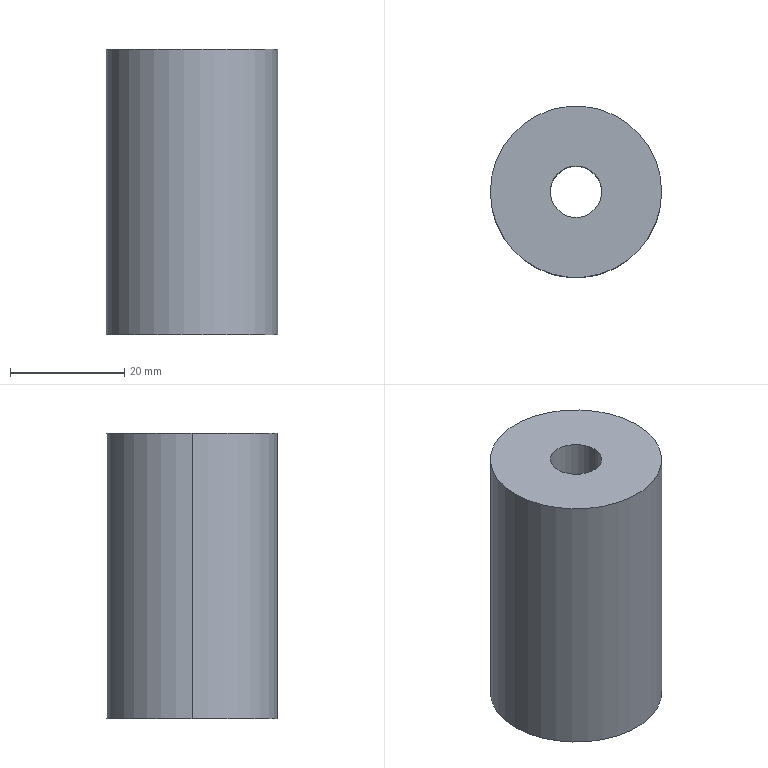Part | SolidWorks | features Extrusion 1 | 1 solid | 6 faces | box 30 x 30 x 50 mm | volume 32162 mm3 | cylinder 4 | plane 2 | commonest cylinder face diameters 9 x2 30 x2
STEP:
#1=CARTESIAN_POINT('',(-4.5,0.,50.));
#2=VERTEX_POINT('',#1);
#3=CARTESIAN_POINT('',(4.5,0.,50.));
#4=VERTEX_POINT('',#3);
#5=CARTESIAN_POINT('',(0.,0.,50.));
#6=DIRECTION('',(0.,0.,1.));
#7=DIRECTION('',(1.,0.,0.));
#8=AXIS2_PLACEMENT_3D('',#5,#6,#7);
#9=CIRCLE('',#8,4.5);
#10=EDGE_CURVE('',#2,#4,#9,.T.);
#11=ORIENTED_EDGE('',*,*,#10,.T.);
#12=CARTESIAN_POINT('',(4.5,0.,0.));
#13=VERTEX_POINT('',#12);
#14=CARTESIAN_POINT('',(4.5,0.,50.));
#15=DIRECTION('',(0.,0.,-1.));
#16=VECTOR('',#15,1000.);
#17=LINE('',#14,#16);
#18=EDGE_CURVE('',#4,#13,#17,.T.);
#19=ORIENTED_EDGE('',*,*,#18,.T.);
#20=CARTESIAN_POINT('',(-4.5,0.,0.));
#21=VERTEX_POINT('',#20);
#22=CARTESIAN_POINT('',(0.,0.,0.));
#23=DIRECTION('',(0.,0.,1.));
#24=DIRECTION('',(1.,0.,0.));
#25=AXIS2_PLACEMENT_3D('',#22,#23,#24);
#26=CIRCLE('',#25,4.5);
#27=EDGE_CURVE('',#21,#13,#26,.T.);
#28=ORIENTED_EDGE('',*,*,#27,.F.);
#29=CARTESIAN_POINT('',(-4.5,0.,50.));
#30=DIRECTION('',(0.,0.,-1.));
#31=VECTOR('',#30,1000.);
#32=LINE('',#29,#31);
#33=EDGE_CURVE('',#2,#21,#32,.T.);
#34=ORIENTED_EDGE('',*,*,#33,.F.);
#35=EDGE_LOOP('',(#11,#19,#28,#34));
#36=FACE_OUTER_BOUND('',#35,.T.);
#37=CARTESIAN_POINT('',(0.,0.,50.));
#38=DIRECTION('',(0.,0.,-1.));
#39=DIRECTION('',(-1.,0.,0.));
#40=AXIS2_PLACEMENT_3D('',#37,#38,#39);
#41=CYLINDRICAL_SURFACE('',#40,4.5);
#42=ADVANCED_FACE('',(#36),#41,.F.);
#43=CARTESIAN_POINT('',(15.,0.,50.));
#44=VERTEX_POINT('',#43);
#45=CARTESIAN_POINT('',(-15.,0.,50.));
#46=VERTEX_POINT('',#45);
#47=CARTESIAN_POINT('',(0.,0.,50.));
#48=DIRECTION('',(0.,0.,1.));
#49=DIRECTION('',(1.,0.,0.));
#50=AXIS2_PLACEMENT_3D('',#47,#48,#49);
#51=CIRCLE('',#50,15.);
#52=EDGE_CURVE('',#44,#46,#51,.T.);
#53=ORIENTED_EDGE('',*,*,#52,.F.);
#54=CARTESIAN_POINT('',(15.,0.,0.));
#55=VERTEX_POINT('',#54);
#56=CARTESIAN_POINT('',(15.,0.,50.));
#57=DIRECTION('',(0.,0.,-1.));
#58=VECTOR('',#57,1000.);
#59=LINE('',#56,#58);
#60=EDGE_CURVE('',#44,#55,#59,.T.);
#61=ORIENTED_EDGE('',*,*,#60,.T.);
#62=CARTESIAN_POINT('',(-15.,0.,0.));
#63=VERTEX_POINT('',#62);
#64=CARTESIAN_POINT('',(0.,0.,0.));
#65=DIRECTION('',(0.,0.,1.));
#66=DIRECTION('',(1.,0.,0.));
#67=AXIS2_PLACEMENT_3D('',#64,#65,#66);
#68=CIRCLE('',#67,15.);
#69=EDGE_CURVE('',#55,#63,#68,.T.);
#70=ORIENTED_EDGE('',*,*,#69,.T.);
#71=CARTESIAN_POINT('',(-15.,0.,50.));
#72=DIRECTION('',(0.,0.,-1.));
#73=VECTOR('',#72,1000.);
#74=LINE('',#71,#73);
#75=EDGE_CURVE('',#46,#63,#74,.T.);
#76=ORIENTED_EDGE('',*,*,#75,.F.);
#77=EDGE_LOOP('',(#53,#61,#70,#76));
#78=FACE_OUTER_BOUND('',#77,.T.);
#79=CARTESIAN_POINT('',(0.,0.,50.));
#80=DIRECTION('',(0.,0.,-1.));
#81=DIRECTION('',(-1.,0.,0.));
#82=AXIS2_PLACEMENT_3D('',#79,#80,#81);
#83=CYLINDRICAL_SURFACE('',#82,15.);
#84=ADVANCED_FACE('',(#78),#83,.T.);
#85=CARTESIAN_POINT('',(0.,0.,50.));
#86=DIRECTION('',(0.,0.,1.));
#87=DIRECTION('',(1.,0.,0.));
#88=AXIS2_PLACEMENT_3D('',#85,#86,#87);
#89=CIRCLE('',#88,15.);
#90=EDGE_CURVE('',#46,#44,#89,.T.);
#91=ORIENTED_EDGE('',*,*,#90,.T.);
#92=ORIENTED_EDGE('',*,*,#52,.T.);
#93=EDGE_LOOP('',(#91,#92));
#94=FACE_OUTER_BOUND('',#93,.T.);
#95=ORIENTED_EDGE('',*,*,#10,.F.);
#96=CARTESIAN_POINT('',(0.,0.,50.));
#97=DIRECTION('',(0.,0.,1.));
#98=DIRECTION('',(1.,0.,0.));
#99=AXIS2_PLACEMENT_3D('',#96,#97,#98);
#100=CIRCLE('',#99,4.5);
#101=EDGE_CURVE('',#4,#2,#100,.T.);
#102=ORIENTED_EDGE('',*,*,#101,.F.);
#103=EDGE_LOOP('',(#95,#102));
#104=FACE_BOUND('',#103,.T.);
#105=CARTESIAN_POINT('',(0.,0.,50.));
#106=DIRECTION('',(0.,0.,1.));
#107=DIRECTION('',(1.,0.,0.));
#108=AXIS2_PLACEMENT_3D('',#105,#106,#107);
#109=PLANE('',#108);
#110=ADVANCED_FACE('',(#94,#104),#109,.T.);
#111=CARTESIAN_POINT('',(0.,0.,0.));
#112=DIRECTION('',(0.,0.,1.));
#113=DIRECTION('',(1.,0.,0.));
#114=AXIS2_PLACEMENT_3D('',#111,#112,#113);
#115=CIRCLE('',#114,15.);
#116=EDGE_CURVE('',#63,#55,#115,.T.);
#117=ORIENTED_EDGE('',*,*,#116,.F.);
#118=ORIENTED_EDGE('',*,*,#69,.F.);
#119=EDGE_LOOP('',(#117,#118));
#120=FACE_OUTER_BOUND('',#119,.T.);
#121=ORIENTED_EDGE('',*,*,#27,.T.);
#122=CARTESIAN_POINT('',(0.,0.,0.));
#123=DIRECTION('',(0.,0.,1.));
#124=DIRECTION('',(1.,0.,0.));
#125=AXIS2_PLACEMENT_3D('',#122,#123,#124);
#126=CIRCLE('',#125,4.5);
#127=EDGE_CURVE('',#13,#21,#126,.T.);
#128=ORIENTED_EDGE('',*,*,#127,.T.);
#129=EDGE_LOOP('',(#121,#128));
#130=FACE_BOUND('',#129,.T.);
#131=CARTESIAN_POINT('',(0.,0.,0.));
#132=DIRECTION('',(0.,0.,1.));
#133=DIRECTION('',(1.,0.,0.));
#134=AXIS2_PLACEMENT_3D('',#131,#132,#133);
#135=PLANE('',#134);
#136=ADVANCED_FACE('',(#120,#130),#135,.F.);
#137=ORIENTED_EDGE('',*,*,#60,.F.);
#138=ORIENTED_EDGE('',*,*,#90,.F.);
#139=ORIENTED_EDGE('',*,*,#75,.T.);
#140=ORIENTED_EDGE('',*,*,#116,.T.);
#141=EDGE_LOOP('',(#137,#138,#139,#140));
#142=FACE_OUTER_BOUND('',#141,.T.);
#143=CARTESIAN_POINT('',(0.,0.,50.));
#144=DIRECTION('',(0.,0.,-1.));
#145=DIRECTION('',(-1.,0.,0.));
#146=AXIS2_PLACEMENT_3D('',#143,#144,#145);
#147=CYLINDRICAL_SURFACE('',#146,15.);
#148=ADVANCED_FACE('',(#142),#147,.T.);
#149=ORIENTED_EDGE('',*,*,#18,.F.);
#150=ORIENTED_EDGE('',*,*,#101,.T.);
#151=ORIENTED_EDGE('',*,*,#33,.T.);
#152=ORIENTED_EDGE('',*,*,#127,.F.);
#153=EDGE_LOOP('',(#149,#150,#151,#152));
#154=FACE_OUTER_BOUND('',#153,.T.);
#155=CARTESIAN_POINT('',(0.,0.,50.));
#156=DIRECTION('',(0.,0.,-1.));
#157=DIRECTION('',(-1.,0.,0.));
#158=AXIS2_PLACEMENT_3D('',#155,#156,#157);
#159=CYLINDRICAL_SURFACE('',#158,4.5);
#160=ADVANCED_FACE('',(#154),#159,.F.);
#161=CLOSED_SHELL('',(#42,#84,#110,#136,#148,#160));
#162=MANIFOLD_SOLID_BREP('',#161);
#163=CARTESIAN_POINT('',(0.,0.,0.));
#164=DIRECTION('',(0.,0.,1.));
#165=DIRECTION('',(1.,0.,0.));
#166=AXIS2_PLACEMENT_3D('',#163,#164,#165);
#167=(LENGTH_UNIT()NAMED_UNIT(*)SI_UNIT(.MILLI.,.METRE.));
#168=UNCERTAINTY_MEASURE_WITH_UNIT(LENGTH_MEASURE(0.00001),#167,'','');
#169=(NAMED_UNIT(*)PLANE_ANGLE_UNIT()SI_UNIT($,.RADIAN.));
#170=(NAMED_UNIT(*)SI_UNIT($,.STERADIAN.)SOLID_ANGLE_UNIT());
#171=(GEOMETRIC_REPRESENTATION_CONTEXT(3)GLOBAL_UNCERTAINTY_ASSIGNED_CONTEXT((#168))GLOBAL_UNIT_ASSIGNED_CONTEXT((#167,#169,#170))REPRESENTATION_CONTEXT('',''));
#172=ADVANCED_BREP_SHAPE_REPRESENTATION('',(#162,#166),#171);